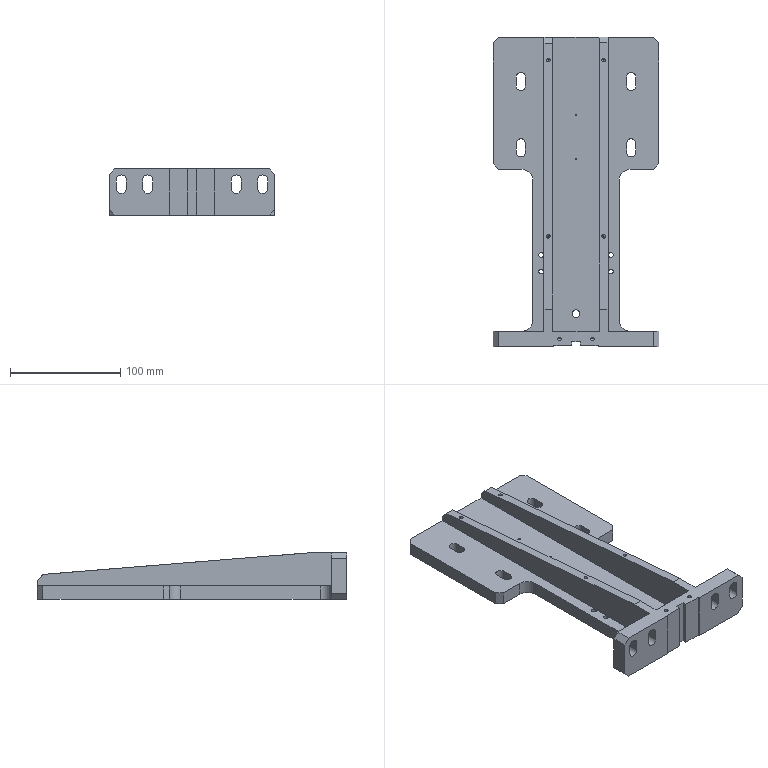Part | SolidWorks | features HoleWzd 8, ICE 7, Chamfer 3, MirrorPattern 3, Extrusion 1, Fillet 1, Rib 1 | 1 solid | 149 faces | box 150 x 280 x 42 mm | volume 505968 mm3 | cylinder 62 | plane 61 | cone 26 | commonest cylinder face diameters 4.2 x14 3.3 x12 9 x12 8.5 x8 6.8 x6 2.5 x4